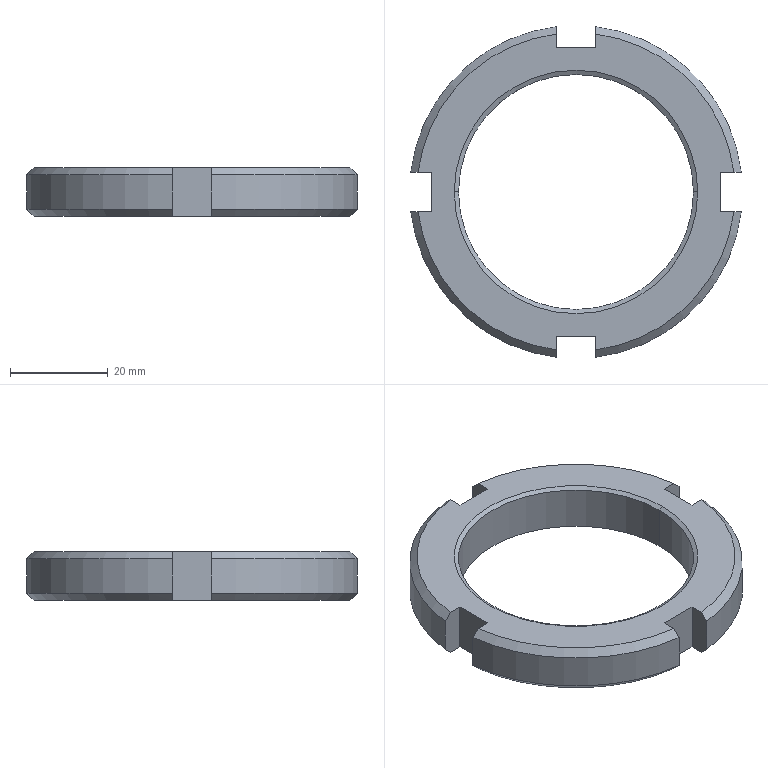Part | STEP file | Round Nut GB/T810-1988 M48x1.5 | 1 solid | 32 faces | box 67.528 x 67.528 x 10 mm | volume 16343 mm3 | plane 14 | cone 12 | cylinder 6 | commonest cylinder face diameters 68 x4 48 x2